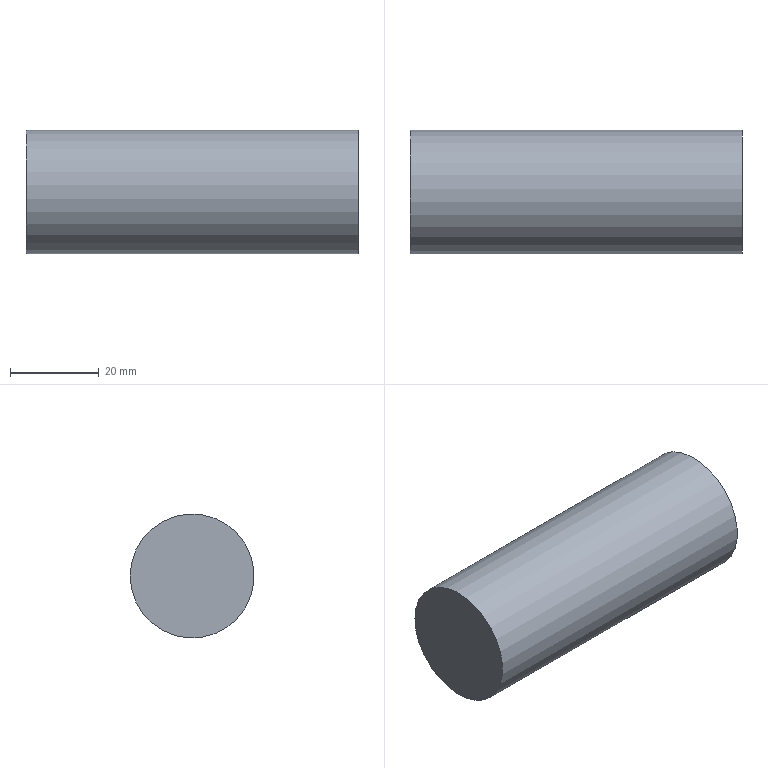Part | NX | features solid 2 | 1 solid | 3 faces | box 75 x 28 x 28 mm | volume 46181 mm3 | plane 2 | cylinder 1 | commonest cylinder face diameters 28 x1
STEP:
#1=CARTESIAN_POINT('',(970.,114.,-330.));
#2=VERTEX_POINT('',#1);
#3=CARTESIAN_POINT('',(970.,100.,-330.));
#4=DIRECTION('',(1.,0.,0.));
#5=DIRECTION('',(0.,1.,0.));
#6=AXIS2_PLACEMENT_3D('',#3,#4,#5);
#7=CIRCLE('',#6,14.);
#8=EDGE_CURVE('',#2,#2,#7,.T.);
#9=ORIENTED_EDGE('',*,*,#8,.F.);
#10=EDGE_LOOP('',(#9));
#11=FACE_BOUND('',#10,.T.);
#12=CARTESIAN_POINT('',(895.,114.,-330.));
#13=VERTEX_POINT('',#12);
#14=CARTESIAN_POINT('',(895.,100.,-330.));
#15=DIRECTION('',(1.,0.,0.));
#16=DIRECTION('',(0.,1.,0.));
#17=AXIS2_PLACEMENT_3D('',#14,#15,#16);
#18=CIRCLE('',#17,14.);
#19=EDGE_CURVE('',#13,#13,#18,.T.);
#20=ORIENTED_EDGE('',*,*,#19,.T.);
#21=EDGE_LOOP('',(#20));
#22=FACE_BOUND('',#21,.T.);
#23=CARTESIAN_POINT('',(970.,100.,-330.));
#24=DIRECTION('',(-1.,0.,0.));
#25=DIRECTION('',(0.,-1.,0.));
#26=AXIS2_PLACEMENT_3D('',#23,#24,#25);
#27=CYLINDRICAL_SURFACE('',#26,14.);
#28=ADVANCED_FACE('',(#11,#22),#27,.T.);
#29=ORIENTED_EDGE('',*,*,#8,.T.);
#30=EDGE_LOOP('',(#29));
#31=FACE_BOUND('',#30,.T.);
#32=CARTESIAN_POINT('',(970.,100.,-330.));
#33=DIRECTION('',(1.,0.,0.));
#34=DIRECTION('',(0.,1.,0.));
#35=AXIS2_PLACEMENT_3D('',#32,#33,#34);
#36=PLANE('',#35);
#37=ADVANCED_FACE('',(#31),#36,.T.);
#38=ORIENTED_EDGE('',*,*,#19,.F.);
#39=EDGE_LOOP('',(#38));
#40=FACE_BOUND('',#39,.T.);
#41=CARTESIAN_POINT('',(895.,100.,-330.));
#42=DIRECTION('',(1.,0.,0.));
#43=DIRECTION('',(0.,1.,0.));
#44=AXIS2_PLACEMENT_3D('',#41,#42,#43);
#45=PLANE('',#44);
#46=ADVANCED_FACE('',(#40),#45,.F.);
#47=CLOSED_SHELL('',(#28,#37,#46));
#48=MANIFOLD_SOLID_BREP('',#47);
#49=(LENGTH_UNIT()NAMED_UNIT(*)SI_UNIT(.MILLI.,.METRE.));
#50=UNCERTAINTY_MEASURE_WITH_UNIT(LENGTH_MEASURE(0.00001),#49,'','');
#51=(NAMED_UNIT(*)PLANE_ANGLE_UNIT()SI_UNIT($,.RADIAN.));
#52=(NAMED_UNIT(*)SI_UNIT($,.STERADIAN.)SOLID_ANGLE_UNIT());
#53=(GEOMETRIC_REPRESENTATION_CONTEXT(3)GLOBAL_UNCERTAINTY_ASSIGNED_CONTEXT((#50))GLOBAL_UNIT_ASSIGNED_CONTEXT((#49,#51,#52))REPRESENTATION_CONTEXT('',''));
#54=ADVANCED_BREP_SHAPE_REPRESENTATION('',(#48),#53);